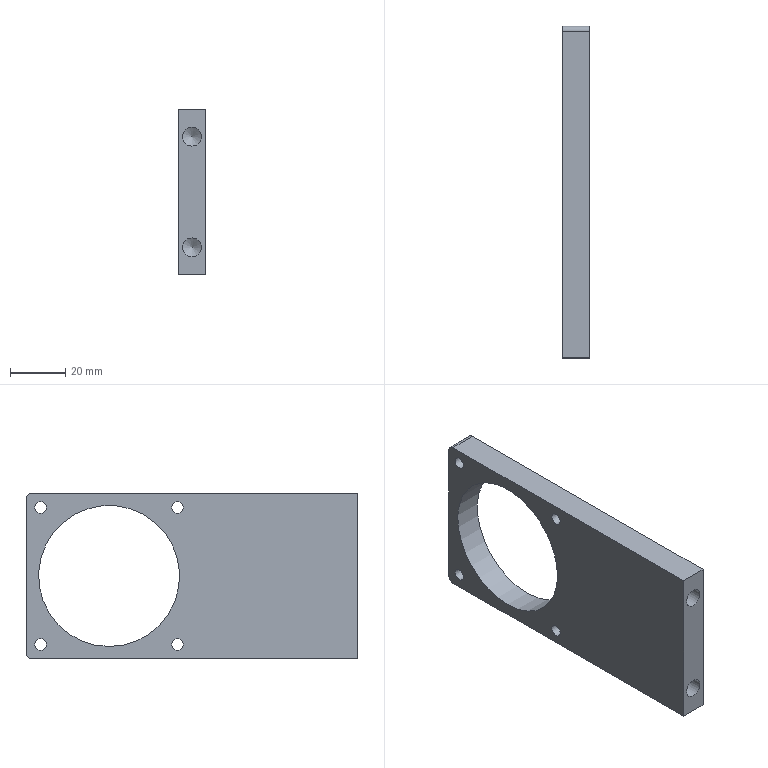Part | STEP file | JBJ-P-1006-03 | 1 solid | 17 faces | box 10 x 120 x 60 mm | volume 49516 mm3 | cylinder 9 | plane 6 | cone 2 | commonest cylinder face diameters 4.2 x4 4 x2 6.8 x2 51 x1
STEP:
#1=CARTESIAN_POINT('',(10.,-2.,0.));
#2=VERTEX_POINT('',#1);
#3=CARTESIAN_POINT('',(10.,-120.,0.));
#4=VERTEX_POINT('',#3);
#5=CARTESIAN_POINT('',(10.,0.,0.));
#6=DIRECTION('',(0.,-1.,0.));
#7=VECTOR('',#6,1000.);
#8=LINE('',#5,#7);
#9=EDGE_CURVE('',#2,#4,#8,.T.);
#10=ORIENTED_EDGE('',*,*,#9,.F.);
#11=CARTESIAN_POINT('',(0.,-2.,0.));
#12=VERTEX_POINT('',#11);
#13=CARTESIAN_POINT('',(10.,-2.,0.));
#14=DIRECTION('',(-1.,0.,0.));
#15=VECTOR('',#14,1000.);
#16=LINE('',#13,#15);
#17=EDGE_CURVE('',#2,#12,#16,.T.);
#18=ORIENTED_EDGE('',*,*,#17,.T.);
#19=CARTESIAN_POINT('',(0.,-120.,0.));
#20=VERTEX_POINT('',#19);
#21=CARTESIAN_POINT('',(0.,0.,0.));
#22=DIRECTION('',(0.,-1.,0.));
#23=VECTOR('',#22,1000.);
#24=LINE('',#21,#23);
#25=EDGE_CURVE('',#12,#20,#24,.T.);
#26=ORIENTED_EDGE('',*,*,#25,.T.);
#27=CARTESIAN_POINT('',(10.,-120.,0.));
#28=DIRECTION('',(-1.,0.,0.));
#29=VECTOR('',#28,1000.);
#30=LINE('',#27,#29);
#31=EDGE_CURVE('',#4,#20,#30,.T.);
#32=ORIENTED_EDGE('',*,*,#31,.F.);
#33=EDGE_LOOP('',(#10,#18,#26,#32));
#34=FACE_OUTER_BOUND('',#33,.T.);
#35=CARTESIAN_POINT('',(10.,0.,0.));
#36=DIRECTION('',(0.,0.,-1.));
#37=DIRECTION('',(0.,1.,0.));
#38=AXIS2_PLACEMENT_3D('',#35,#36,#37);
#39=PLANE('',#38);
#40=ADVANCED_FACE('',(#34),#39,.F.);
#41=CARTESIAN_POINT('',(5.,-120.,-13.4));
#42=VERTEX_POINT('',#41);
#43=CARTESIAN_POINT('',(5.,-120.,-10.));
#44=DIRECTION('',(0.,-1.,0.));
#45=DIRECTION('',(0.,0.,-1.));
#46=AXIS2_PLACEMENT_3D('',#43,#44,#45);
#47=CIRCLE('',#46,3.4);
#48=EDGE_CURVE('',#42,#42,#47,.T.);
#49=ORIENTED_EDGE('',*,*,#48,.F.);
#50=EDGE_LOOP('',(#49));
#51=FACE_BOUND('',#50,.T.);
#52=CARTESIAN_POINT('',(5.,-120.,-53.4));
#53=VERTEX_POINT('',#52);
#54=CARTESIAN_POINT('',(5.,-120.,-50.));
#55=DIRECTION('',(0.,-1.,0.));
#56=DIRECTION('',(0.,0.,-1.));
#57=AXIS2_PLACEMENT_3D('',#54,#55,#56);
#58=CIRCLE('',#57,3.4);
#59=EDGE_CURVE('',#53,#53,#58,.T.);
#60=ORIENTED_EDGE('',*,*,#59,.F.);
#61=EDGE_LOOP('',(#60));
#62=FACE_BOUND('',#61,.T.);
#63=CARTESIAN_POINT('',(0.,-120.,-60.));
#64=VERTEX_POINT('',#63);
#65=CARTESIAN_POINT('',(0.,-120.,0.));
#66=DIRECTION('',(0.,0.,-1.));
#67=VECTOR('',#66,1000.);
#68=LINE('',#65,#67);
#69=EDGE_CURVE('',#20,#64,#68,.T.);
#70=ORIENTED_EDGE('',*,*,#69,.T.);
#71=CARTESIAN_POINT('',(10.,-120.,-60.));
#72=VERTEX_POINT('',#71);
#73=CARTESIAN_POINT('',(10.,-120.,-60.));
#74=DIRECTION('',(-1.,0.,0.));
#75=VECTOR('',#74,1000.);
#76=LINE('',#73,#75);
#77=EDGE_CURVE('',#72,#64,#76,.T.);
#78=ORIENTED_EDGE('',*,*,#77,.F.);
#79=CARTESIAN_POINT('',(10.,-120.,0.));
#80=DIRECTION('',(0.,0.,-1.));
#81=VECTOR('',#80,1000.);
#82=LINE('',#79,#81);
#83=EDGE_CURVE('',#4,#72,#82,.T.);
#84=ORIENTED_EDGE('',*,*,#83,.F.);
#85=ORIENTED_EDGE('',*,*,#31,.T.);
#86=EDGE_LOOP('',(#70,#78,#84,#85));
#87=FACE_OUTER_BOUND('',#86,.T.);
#88=CARTESIAN_POINT('',(10.,-120.,0.));
#89=DIRECTION('',(0.,1.,0.));
#90=DIRECTION('',(0.,0.,1.));
#91=AXIS2_PLACEMENT_3D('',#88,#89,#90);
#92=PLANE('',#91);
#93=ADVANCED_FACE('',(#51,#62,#87),#92,.F.);
#94=CARTESIAN_POINT('',(0.,-2.,-60.));
#95=VERTEX_POINT('',#94);
#96=CARTESIAN_POINT('',(0.,0.,-60.));
#97=DIRECTION('',(0.,1.,0.));
#98=VECTOR('',#97,1000.);
#99=LINE('',#96,#98);
#100=EDGE_CURVE('',#64,#95,#99,.T.);
#101=ORIENTED_EDGE('',*,*,#100,.T.);
#102=CARTESIAN_POINT('',(10.,-2.,-60.));
#103=VERTEX_POINT('',#102);
#104=CARTESIAN_POINT('',(10.,-2.,-60.));
#105=DIRECTION('',(1.,0.,0.));
#106=VECTOR('',#105,1000.);
#107=LINE('',#104,#106);
#108=EDGE_CURVE('',#95,#103,#107,.T.);
#109=ORIENTED_EDGE('',*,*,#108,.T.);
#110=CARTESIAN_POINT('',(10.,0.,-60.));
#111=DIRECTION('',(0.,1.,0.));
#112=VECTOR('',#111,1000.);
#113=LINE('',#110,#112);
#114=EDGE_CURVE('',#72,#103,#113,.T.);
#115=ORIENTED_EDGE('',*,*,#114,.F.);
#116=ORIENTED_EDGE('',*,*,#77,.T.);
#117=EDGE_LOOP('',(#101,#109,#115,#116));
#118=FACE_OUTER_BOUND('',#117,.T.);
#119=CARTESIAN_POINT('',(10.,0.,-60.));
#120=DIRECTION('',(0.,0.,1.));
#121=DIRECTION('',(0.,-1.,0.));
#122=AXIS2_PLACEMENT_3D('',#119,#120,#121);
#123=PLANE('',#122);
#124=ADVANCED_FACE('',(#118),#123,.F.);
#125=CARTESIAN_POINT('',(0.,0.,-58.));
#126=VERTEX_POINT('',#125);
#127=CARTESIAN_POINT('',(0.,0.,-2.));
#128=VERTEX_POINT('',#127);
#129=CARTESIAN_POINT('',(0.,0.,0.));
#130=DIRECTION('',(0.,0.,1.));
#131=VECTOR('',#130,1000.);
#132=LINE('',#129,#131);
#133=EDGE_CURVE('',#126,#128,#132,.T.);
#134=ORIENTED_EDGE('',*,*,#133,.T.);
#135=CARTESIAN_POINT('',(10.,0.,-2.));
#136=VERTEX_POINT('',#135);
#137=CARTESIAN_POINT('',(10.,0.,-2.));
#138=DIRECTION('',(1.,0.,0.));
#139=VECTOR('',#138,1000.);
#140=LINE('',#137,#139);
#141=EDGE_CURVE('',#128,#136,#140,.T.);
#142=ORIENTED_EDGE('',*,*,#141,.T.);
#143=CARTESIAN_POINT('',(10.,0.,-58.));
#144=VERTEX_POINT('',#143);
#145=CARTESIAN_POINT('',(10.,0.,0.));
#146=DIRECTION('',(0.,0.,1.));
#147=VECTOR('',#146,1000.);
#148=LINE('',#145,#147);
#149=EDGE_CURVE('',#144,#136,#148,.T.);
#150=ORIENTED_EDGE('',*,*,#149,.F.);
#151=CARTESIAN_POINT('',(10.,0.,-58.));
#152=DIRECTION('',(-1.,0.,0.));
#153=VECTOR('',#152,1000.);
#154=LINE('',#151,#153);
#155=EDGE_CURVE('',#144,#126,#154,.T.);
#156=ORIENTED_EDGE('',*,*,#155,.T.);
#157=EDGE_LOOP('',(#134,#142,#150,#156));
#158=FACE_OUTER_BOUND('',#157,.T.);
#159=CARTESIAN_POINT('',(10.,0.,0.));
#160=DIRECTION('',(0.,-1.,0.));
#161=DIRECTION('',(0.,0.,-1.));
#162=AXIS2_PLACEMENT_3D('',#159,#160,#161);
#163=PLANE('',#162);
#164=ADVANCED_FACE('',(#158),#163,.F.);
#165=CARTESIAN_POINT('',(10.,-30.003,-55.5));
#166=VERTEX_POINT('',#165);
#167=CARTESIAN_POINT('',(10.,-30.003,-30.));
#168=DIRECTION('',(1.,0.,0.));
#169=DIRECTION('',(0.,0.,-1.));
#170=AXIS2_PLACEMENT_3D('',#167,#168,#169);
#171=CIRCLE('',#170,25.5);
#172=EDGE_CURVE('',#166,#166,#171,.T.);
#173=ORIENTED_EDGE('',*,*,#172,.F.);
#174=EDGE_LOOP('',(#173));
#175=FACE_BOUND('',#174,.T.);
#176=CARTESIAN_POINT('',(10.,-5.251,-52.649));
#177=VERTEX_POINT('',#176);
#178=CARTESIAN_POINT('',(10.,-5.251,-54.749));
#179=DIRECTION('',(-1.,0.,0.));
#180=DIRECTION('',(0.,0.,1.));
#181=AXIS2_PLACEMENT_3D('',#178,#179,#180);
#182=CIRCLE('',#181,2.1);
#183=EDGE_CURVE('',#177,#177,#182,.T.);
#184=ORIENTED_EDGE('',*,*,#183,.T.);
#185=EDGE_LOOP('',(#184));
#186=FACE_BOUND('',#185,.T.);
#187=CARTESIAN_POINT('',(10.,-5.251,-3.151));
#188=VERTEX_POINT('',#187);
#189=CARTESIAN_POINT('',(10.,-5.251,-5.251));
#190=DIRECTION('',(-1.,0.,0.));
#191=DIRECTION('',(0.,0.,1.));
#192=AXIS2_PLACEMENT_3D('',#189,#190,#191);
#193=CIRCLE('',#192,2.1);
#194=EDGE_CURVE('',#188,#188,#193,.T.);
#195=ORIENTED_EDGE('',*,*,#194,.T.);
#196=EDGE_LOOP('',(#195));
#197=FACE_BOUND('',#196,.T.);
#198=CARTESIAN_POINT('',(10.,-54.749,-3.151));
#199=VERTEX_POINT('',#198);
#200=CARTESIAN_POINT('',(10.,-54.749,-5.251));
#201=DIRECTION('',(-1.,0.,0.));
#202=DIRECTION('',(0.,0.,1.));
#203=AXIS2_PLACEMENT_3D('',#200,#201,#202);
#204=CIRCLE('',#203,2.1);
#205=EDGE_CURVE('',#199,#199,#204,.T.);
#206=ORIENTED_EDGE('',*,*,#205,.T.);
#207=EDGE_LOOP('',(#206));
#208=FACE_BOUND('',#207,.T.);
#209=CARTESIAN_POINT('',(10.,-54.749,-52.649));
#210=VERTEX_POINT('',#209);
#211=CARTESIAN_POINT('',(10.,-54.749,-54.749));
#212=DIRECTION('',(-1.,0.,0.));
#213=DIRECTION('',(0.,0.,1.));
#214=AXIS2_PLACEMENT_3D('',#211,#212,#213);
#215=CIRCLE('',#214,2.1);
#216=EDGE_CURVE('',#210,#210,#215,.T.);
#217=ORIENTED_EDGE('',*,*,#216,.T.);
#218=EDGE_LOOP('',(#217));
#219=FACE_BOUND('',#218,.T.);
#220=ORIENTED_EDGE('',*,*,#149,.T.);
#221=CARTESIAN_POINT('',(10.,-2.,-2.));
#222=DIRECTION('',(1.,0.,0.));
#223=DIRECTION('',(0.,0.,-1.));
#224=AXIS2_PLACEMENT_3D('',#221,#222,#223);
#225=CIRCLE('',#224,2.);
#226=EDGE_CURVE('',#136,#2,#225,.T.);
#227=ORIENTED_EDGE('',*,*,#226,.T.);
#228=ORIENTED_EDGE('',*,*,#9,.T.);
#229=ORIENTED_EDGE('',*,*,#83,.T.);
#230=ORIENTED_EDGE('',*,*,#114,.T.);
#231=CARTESIAN_POINT('',(10.,-2.,-58.));
#232=DIRECTION('',(1.,0.,0.));
#233=DIRECTION('',(0.,0.,-1.));
#234=AXIS2_PLACEMENT_3D('',#231,#232,#233);
#235=CIRCLE('',#234,2.);
#236=EDGE_CURVE('',#103,#144,#235,.T.);
#237=ORIENTED_EDGE('',*,*,#236,.T.);
#238=EDGE_LOOP('',(#220,#227,#228,#229,#230,#237));
#239=FACE_OUTER_BOUND('',#238,.T.);
#240=CARTESIAN_POINT('',(10.,0.,0.));
#241=DIRECTION('',(1.,0.,0.));
#242=DIRECTION('',(0.,0.,-1.));
#243=AXIS2_PLACEMENT_3D('',#240,#241,#242);
#244=PLANE('',#243);
#245=ADVANCED_FACE('',(#175,#186,#197,#208,#219,#239),#244,.T.);
#246=CARTESIAN_POINT('',(0.,-30.003,-55.5));
#247=VERTEX_POINT('',#246);
#248=CARTESIAN_POINT('',(0.,-30.003,-30.));
#249=DIRECTION('',(1.,0.,0.));
#250=DIRECTION('',(0.,0.,-1.));
#251=AXIS2_PLACEMENT_3D('',#248,#249,#250);
#252=CIRCLE('',#251,25.5);
#253=EDGE_CURVE('',#247,#247,#252,.T.);
#254=ORIENTED_EDGE('',*,*,#253,.T.);
#255=EDGE_LOOP('',(#254));
#256=FACE_BOUND('',#255,.T.);
#257=CARTESIAN_POINT('',(0.,-5.251,-52.649));
#258=VERTEX_POINT('',#257);
#259=CARTESIAN_POINT('',(0.,-5.251,-54.749));
#260=DIRECTION('',(-1.,0.,0.));
#261=DIRECTION('',(0.,0.,1.));
#262=AXIS2_PLACEMENT_3D('',#259,#260,#261);
#263=CIRCLE('',#262,2.1);
#264=EDGE_CURVE('',#258,#258,#263,.T.);
#265=ORIENTED_EDGE('',*,*,#264,.F.);
#266=EDGE_LOOP('',(#265));
#267=FACE_BOUND('',#266,.T.);
#268=CARTESIAN_POINT('',(0.,-5.251,-3.151));
#269=VERTEX_POINT('',#268);
#270=CARTESIAN_POINT('',(0.,-5.251,-5.251));
#271=DIRECTION('',(-1.,0.,0.));
#272=DIRECTION('',(0.,0.,1.));
#273=AXIS2_PLACEMENT_3D('',#270,#271,#272);
#274=CIRCLE('',#273,2.1);
#275=EDGE_CURVE('',#269,#269,#274,.T.);
#276=ORIENTED_EDGE('',*,*,#275,.F.);
#277=EDGE_LOOP('',(#276));
#278=FACE_BOUND('',#277,.T.);
#279=CARTESIAN_POINT('',(0.,-54.749,-3.151));
#280=VERTEX_POINT('',#279);
#281=CARTESIAN_POINT('',(0.,-54.749,-5.251));
#282=DIRECTION('',(-1.,0.,0.));
#283=DIRECTION('',(0.,0.,1.));
#284=AXIS2_PLACEMENT_3D('',#281,#282,#283);
#285=CIRCLE('',#284,2.1);
#286=EDGE_CURVE('',#280,#280,#285,.T.);
#287=ORIENTED_EDGE('',*,*,#286,.F.);
#288=EDGE_LOOP('',(#287));
#289=FACE_BOUND('',#288,.T.);
#290=CARTESIAN_POINT('',(0.,-54.749,-52.649));
#291=VERTEX_POINT('',#290);
#292=CARTESIAN_POINT('',(0.,-54.749,-54.749));
#293=DIRECTION('',(-1.,0.,0.));
#294=DIRECTION('',(0.,0.,1.));
#295=AXIS2_PLACEMENT_3D('',#292,#293,#294);
#296=CIRCLE('',#295,2.1);
#297=EDGE_CURVE('',#291,#291,#296,.T.);
#298=ORIENTED_EDGE('',*,*,#297,.F.);
#299=EDGE_LOOP('',(#298));
#300=FACE_BOUND('',#299,.T.);
#301=ORIENTED_EDGE('',*,*,#25,.F.);
#302=CARTESIAN_POINT('',(0.,-2.,-2.));
#303=DIRECTION('',(-1.,0.,0.));
#304=DIRECTION('',(0.,0.,-1.));
#305=AXIS2_PLACEMENT_3D('',#302,#303,#304);
#306=CIRCLE('',#305,2.);
#307=EDGE_CURVE('',#12,#128,#306,.T.);
#308=ORIENTED_EDGE('',*,*,#307,.T.);
#309=ORIENTED_EDGE('',*,*,#133,.F.);
#310=CARTESIAN_POINT('',(0.,-2.,-58.));
#311=DIRECTION('',(-1.,0.,0.));
#312=DIRECTION('',(0.,0.,-1.));
#313=AXIS2_PLACEMENT_3D('',#310,#311,#312);
#314=CIRCLE('',#313,2.);
#315=EDGE_CURVE('',#126,#95,#314,.T.);
#316=ORIENTED_EDGE('',*,*,#315,.T.);
#317=ORIENTED_EDGE('',*,*,#100,.F.);
#318=ORIENTED_EDGE('',*,*,#69,.F.);
#319=EDGE_LOOP('',(#301,#308,#309,#316,#317,#318));
#320=FACE_OUTER_BOUND('',#319,.T.);
#321=CARTESIAN_POINT('',(0.,0.,0.));
#322=DIRECTION('',(1.,0.,0.));
#323=DIRECTION('',(0.,0.,-1.));
#324=AXIS2_PLACEMENT_3D('',#321,#322,#323);
#325=PLANE('',#324);
#326=ADVANCED_FACE('',(#256,#267,#278,#289,#300,#320),#325,.F.);
#327=ORIENTED_EDGE('',*,*,#216,.F.);
#328=EDGE_LOOP('',(#327));
#329=FACE_OUTER_BOUND('',#328,.T.);
#330=ORIENTED_EDGE('',*,*,#297,.T.);
#331=EDGE_LOOP('',(#330));
#332=FACE_OUTER_BOUND('',#331,.T.);
#333=CARTESIAN_POINT('',(0.,-54.749,-54.749));
#334=DIRECTION('',(-1.,0.,0.));
#335=DIRECTION('',(0.,0.,1.));
#336=AXIS2_PLACEMENT_3D('',#333,#334,#335);
#337=CYLINDRICAL_SURFACE('',#336,2.1);
#338=ADVANCED_FACE('',(#329,#332),#337,.F.);
#339=ORIENTED_EDGE('',*,*,#205,.F.);
#340=EDGE_LOOP('',(#339));
#341=FACE_OUTER_BOUND('',#340,.T.);
#342=ORIENTED_EDGE('',*,*,#286,.T.);
#343=EDGE_LOOP('',(#342));
#344=FACE_OUTER_BOUND('',#343,.T.);
#345=CARTESIAN_POINT('',(0.,-54.749,-5.251));
#346=DIRECTION('',(-1.,0.,0.));
#347=DIRECTION('',(0.,0.,1.));
#348=AXIS2_PLACEMENT_3D('',#345,#346,#347);
#349=CYLINDRICAL_SURFACE('',#348,2.1);
#350=ADVANCED_FACE('',(#341,#344),#349,.F.);
#351=ORIENTED_EDGE('',*,*,#194,.F.);
#352=EDGE_LOOP('',(#351));
#353=FACE_OUTER_BOUND('',#352,.T.);
#354=ORIENTED_EDGE('',*,*,#275,.T.);
#355=EDGE_LOOP('',(#354));
#356=FACE_OUTER_BOUND('',#355,.T.);
#357=CARTESIAN_POINT('',(0.,-5.251,-5.251));
#358=DIRECTION('',(-1.,0.,0.));
#359=DIRECTION('',(0.,0.,1.));
#360=AXIS2_PLACEMENT_3D('',#357,#358,#359);
#361=CYLINDRICAL_SURFACE('',#360,2.1);
#362=ADVANCED_FACE('',(#353,#356),#361,.F.);
#363=ORIENTED_EDGE('',*,*,#183,.F.);
#364=EDGE_LOOP('',(#363));
#365=FACE_OUTER_BOUND('',#364,.T.);
#366=ORIENTED_EDGE('',*,*,#264,.T.);
#367=EDGE_LOOP('',(#366));
#368=FACE_OUTER_BOUND('',#367,.T.);
#369=CARTESIAN_POINT('',(0.,-5.251,-54.749));
#370=DIRECTION('',(-1.,0.,0.));
#371=DIRECTION('',(0.,0.,1.));
#372=AXIS2_PLACEMENT_3D('',#369,#370,#371);
#373=CYLINDRICAL_SURFACE('',#372,2.1);
#374=ADVANCED_FACE('',(#365,#368),#373,.F.);
#375=ORIENTED_EDGE('',*,*,#253,.F.);
#376=EDGE_LOOP('',(#375));
#377=FACE_OUTER_BOUND('',#376,.T.);
#378=ORIENTED_EDGE('',*,*,#172,.T.);
#379=EDGE_LOOP('',(#378));
#380=FACE_OUTER_BOUND('',#379,.T.);
#381=CARTESIAN_POINT('',(0.,-30.003,-30.));
#382=DIRECTION('',(1.,0.,0.));
#383=DIRECTION('',(0.,0.,-1.));
#384=AXIS2_PLACEMENT_3D('',#381,#382,#383);
#385=CYLINDRICAL_SURFACE('',#384,25.5);
#386=ADVANCED_FACE('',(#377,#380),#385,.F.);
#387=CARTESIAN_POINT('',(5.,-100.25,-53.4));
#388=VERTEX_POINT('',#387);
#389=CARTESIAN_POINT('',(5.,-100.25,-50.));
#390=DIRECTION('',(0.,-1.,0.));
#391=DIRECTION('',(0.,0.,-1.));
#392=AXIS2_PLACEMENT_3D('',#389,#390,#391);
#393=CIRCLE('',#392,3.4);
#394=EDGE_CURVE('',#388,#388,#393,.T.);
#395=ORIENTED_EDGE('',*,*,#394,.T.);
#396=EDGE_LOOP('',(#395));
#397=FACE_OUTER_BOUND('',#396,.T.);
#398=CARTESIAN_POINT('',(5.,-100.25,-50.));
#399=DIRECTION('',(0.,-1.,0.));
#400=DIRECTION('',(0.,0.,-1.));
#401=AXIS2_PLACEMENT_3D('',#398,#399,#400);
#402=CONICAL_SURFACE('',#401,3.4,1.03);
#403=ADVANCED_FACE('',(#397),#402,.F.);
#404=ORIENTED_EDGE('',*,*,#394,.F.);
#405=EDGE_LOOP('',(#404));
#406=FACE_OUTER_BOUND('',#405,.T.);
#407=ORIENTED_EDGE('',*,*,#59,.T.);
#408=EDGE_LOOP('',(#407));
#409=FACE_OUTER_BOUND('',#408,.T.);
#410=CARTESIAN_POINT('',(5.,-120.,-50.));
#411=DIRECTION('',(0.,-1.,0.));
#412=DIRECTION('',(0.,0.,-1.));
#413=AXIS2_PLACEMENT_3D('',#410,#411,#412);
#414=CYLINDRICAL_SURFACE('',#413,3.4);
#415=ADVANCED_FACE('',(#406,#409),#414,.F.);
#416=CARTESIAN_POINT('',(5.,-100.25,-13.4));
#417=VERTEX_POINT('',#416);
#418=CARTESIAN_POINT('',(5.,-100.25,-10.));
#419=DIRECTION('',(0.,-1.,0.));
#420=DIRECTION('',(0.,0.,-1.));
#421=AXIS2_PLACEMENT_3D('',#418,#419,#420);
#422=CIRCLE('',#421,3.4);
#423=EDGE_CURVE('',#417,#417,#422,.T.);
#424=ORIENTED_EDGE('',*,*,#423,.T.);
#425=EDGE_LOOP('',(#424));
#426=FACE_OUTER_BOUND('',#425,.T.);
#427=CARTESIAN_POINT('',(5.,-100.25,-10.));
#428=DIRECTION('',(0.,-1.,0.));
#429=DIRECTION('',(0.,0.,-1.));
#430=AXIS2_PLACEMENT_3D('',#427,#428,#429);
#431=CONICAL_SURFACE('',#430,3.4,1.03);
#432=ADVANCED_FACE('',(#426),#431,.F.);
#433=ORIENTED_EDGE('',*,*,#423,.F.);
#434=EDGE_LOOP('',(#433));
#435=FACE_OUTER_BOUND('',#434,.T.);
#436=ORIENTED_EDGE('',*,*,#48,.T.);
#437=EDGE_LOOP('',(#436));
#438=FACE_OUTER_BOUND('',#437,.T.);
#439=CARTESIAN_POINT('',(5.,-120.,-10.));
#440=DIRECTION('',(0.,-1.,0.));
#441=DIRECTION('',(0.,0.,-1.));
#442=AXIS2_PLACEMENT_3D('',#439,#440,#441);
#443=CYLINDRICAL_SURFACE('',#442,3.4);
#444=ADVANCED_FACE('',(#435,#438),#443,.F.);
#445=ORIENTED_EDGE('',*,*,#226,.F.);
#446=ORIENTED_EDGE('',*,*,#141,.F.);
#447=ORIENTED_EDGE('',*,*,#307,.F.);
#448=ORIENTED_EDGE('',*,*,#17,.F.);
#449=EDGE_LOOP('',(#445,#446,#447,#448));
#450=FACE_OUTER_BOUND('',#449,.T.);
#451=CARTESIAN_POINT('',(10.,-2.,-2.));
#452=DIRECTION('',(-1.,0.,0.));
#453=DIRECTION('',(0.,0.,1.));
#454=AXIS2_PLACEMENT_3D('',#451,#452,#453);
#455=CYLINDRICAL_SURFACE('',#454,2.);
#456=ADVANCED_FACE('',(#450),#455,.T.);
#457=ORIENTED_EDGE('',*,*,#236,.F.);
#458=ORIENTED_EDGE('',*,*,#108,.F.);
#459=ORIENTED_EDGE('',*,*,#315,.F.);
#460=ORIENTED_EDGE('',*,*,#155,.F.);
#461=EDGE_LOOP('',(#457,#458,#459,#460));
#462=FACE_OUTER_BOUND('',#461,.T.);
#463=CARTESIAN_POINT('',(10.,-2.,-58.));
#464=DIRECTION('',(-1.,0.,0.));
#465=DIRECTION('',(0.,0.,1.));
#466=AXIS2_PLACEMENT_3D('',#463,#464,#465);
#467=CYLINDRICAL_SURFACE('',#466,2.);
#468=ADVANCED_FACE('',(#462),#467,.T.);
#469=CLOSED_SHELL('',(#40,#93,#124,#164,#245,#326,#338,#350,#362,#374,#386,#403,#415,#432,#444,#456,#468));
#470=MANIFOLD_SOLID_BREP('',#469);
#471=CARTESIAN_POINT('',(0.,0.,0.));
#472=DIRECTION('',(0.,0.,1.));
#473=DIRECTION('',(1.,0.,0.));
#474=AXIS2_PLACEMENT_3D('',#471,#472,#473);
#475=(LENGTH_UNIT()NAMED_UNIT(*)SI_UNIT(.MILLI.,.METRE.));
#476=UNCERTAINTY_MEASURE_WITH_UNIT(LENGTH_MEASURE(0.00001),#475,'','');
#477=(NAMED_UNIT(*)PLANE_ANGLE_UNIT()SI_UNIT($,.RADIAN.));
#478=(NAMED_UNIT(*)SI_UNIT($,.STERADIAN.)SOLID_ANGLE_UNIT());
#479=(GEOMETRIC_REPRESENTATION_CONTEXT(3)GLOBAL_UNCERTAINTY_ASSIGNED_CONTEXT((#476))GLOBAL_UNIT_ASSIGNED_CONTEXT((#475,#477,#478))REPRESENTATION_CONTEXT('',''));
#480=ADVANCED_BREP_SHAPE_REPRESENTATION('',(#470,#474),#479);